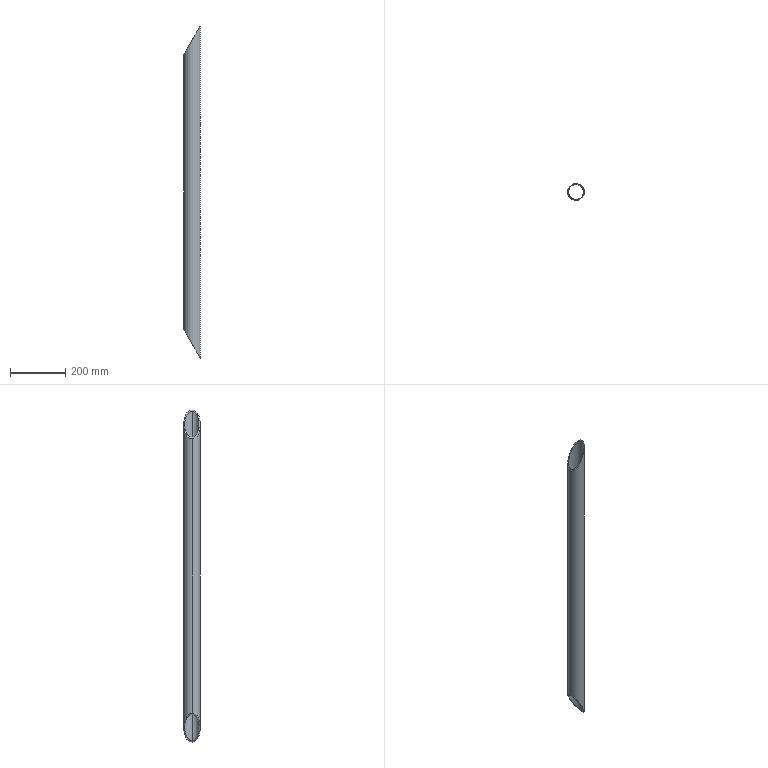Part | SolidWorks | features BaseBody 1, HoleWzd 1 | 1 solid | 6 faces | box 60.3 x 60.3 x 1200 mm | volume 628920 mm3 | cylinder 4 | plane 2 | commonest cylinder face diameters 53.9 x2 60.3 x2
STEP:
#1=CARTESIAN_POINT('',(-26.95,0.,-501.1));
#2=VERTEX_POINT('',#1);
#3=CARTESIAN_POINT('',(26.95,0.,-594.457));
#4=VERTEX_POINT('',#3);
#5=CARTESIAN_POINT('',(-26.95,0.,-501.1));
#6=CARTESIAN_POINT('',(-26.95,-53.9,-501.1));
#7=CARTESIAN_POINT('',(26.95,-53.9,-594.457));
#8=CARTESIAN_POINT('',(26.95,0.,-594.457));
#9=(BOUNDED_CURVE()B_SPLINE_CURVE(3,(#5,#6,#7,#8),.UNSPECIFIED.,.F.,.T.)B_SPLINE_CURVE_WITH_KNOTS((4,4),(0.,3.142),.UNSPECIFIED.)CURVE()GEOMETRIC_REPRESENTATION_ITEM()RATIONAL_B_SPLINE_CURVE((1.,0.3333,0.3333,1.))REPRESENTATION_ITEM(''));
#10=EDGE_CURVE('',#2,#4,#9,.T.);
#11=ORIENTED_EDGE('',*,*,#10,.F.);
#12=CARTESIAN_POINT('',(-26.95,0.,501.1));
#13=VERTEX_POINT('',#12);
#14=CARTESIAN_POINT('',(-26.95,0.,597.229));
#15=DIRECTION('',(0.,0.,1.));
#16=VECTOR('',#15,1000.);
#17=LINE('',#14,#16);
#18=EDGE_CURVE('',#2,#13,#17,.T.);
#19=ORIENTED_EDGE('',*,*,#18,.T.);
#20=CARTESIAN_POINT('',(26.95,0.,594.457));
#21=VERTEX_POINT('',#20);
#22=CARTESIAN_POINT('',(-26.95,0.,501.1));
#23=CARTESIAN_POINT('',(-26.95,-53.9,501.1));
#24=CARTESIAN_POINT('',(26.95,-53.9,594.457));
#25=CARTESIAN_POINT('',(26.95,0.,594.457));
#26=(BOUNDED_CURVE()B_SPLINE_CURVE(3,(#22,#23,#24,#25),.UNSPECIFIED.,.F.,.T.)B_SPLINE_CURVE_WITH_KNOTS((4,4),(3.142,6.283),.UNSPECIFIED.)CURVE()GEOMETRIC_REPRESENTATION_ITEM()RATIONAL_B_SPLINE_CURVE((1.,0.3333,0.3333,1.))REPRESENTATION_ITEM(''));
#27=EDGE_CURVE('',#13,#21,#26,.T.);
#28=ORIENTED_EDGE('',*,*,#27,.T.);
#29=CARTESIAN_POINT('',(26.95,0.,597.229));
#30=DIRECTION('',(0.,0.,1.));
#31=VECTOR('',#30,1000.);
#32=LINE('',#29,#31);
#33=EDGE_CURVE('',#4,#21,#32,.T.);
#34=ORIENTED_EDGE('',*,*,#33,.F.);
#35=EDGE_LOOP('',(#11,#19,#28,#34));
#36=FACE_OUTER_BOUND('',#35,.T.);
#37=CARTESIAN_POINT('',(0.,0.,597.229));
#38=DIRECTION('',(0.,0.,1.));
#39=DIRECTION('',(1.,0.,0.));
#40=AXIS2_PLACEMENT_3D('',#37,#38,#39);
#41=CYLINDRICAL_SURFACE('',#40,26.95);
#42=ADVANCED_FACE('',(#36),#41,.F.);
#43=CARTESIAN_POINT('',(30.15,0.,600.));
#44=VERTEX_POINT('',#43);
#45=CARTESIAN_POINT('',(-30.15,0.,495.557));
#46=VERTEX_POINT('',#45);
#47=CARTESIAN_POINT('',(30.15,0.,600.));
#48=CARTESIAN_POINT('',(30.15,60.3,600.));
#49=CARTESIAN_POINT('',(-30.15,60.3,495.557));
#50=CARTESIAN_POINT('',(-30.15,0.,495.557));
#51=(BOUNDED_CURVE()B_SPLINE_CURVE(3,(#47,#48,#49,#50),.UNSPECIFIED.,.F.,.T.)B_SPLINE_CURVE_WITH_KNOTS((4,4),(3.142,6.283),.UNSPECIFIED.)CURVE()GEOMETRIC_REPRESENTATION_ITEM()RATIONAL_B_SPLINE_CURVE((1.,0.3333,0.3333,1.))REPRESENTATION_ITEM(''));
#52=EDGE_CURVE('',#44,#46,#51,.T.);
#53=ORIENTED_EDGE('',*,*,#52,.F.);
#54=CARTESIAN_POINT('',(30.15,0.,-600.));
#55=VERTEX_POINT('',#54);
#56=CARTESIAN_POINT('',(30.15,0.,600.));
#57=DIRECTION('',(0.,0.,-1.));
#58=VECTOR('',#57,1000.);
#59=LINE('',#56,#58);
#60=EDGE_CURVE('',#44,#55,#59,.T.);
#61=ORIENTED_EDGE('',*,*,#60,.T.);
#62=CARTESIAN_POINT('',(-30.15,0.,-495.557));
#63=VERTEX_POINT('',#62);
#64=CARTESIAN_POINT('',(30.15,0.,-600.));
#65=CARTESIAN_POINT('',(30.15,60.3,-600.));
#66=CARTESIAN_POINT('',(-30.15,60.3,-495.557));
#67=CARTESIAN_POINT('',(-30.15,0.,-495.557));
#68=(BOUNDED_CURVE()B_SPLINE_CURVE(3,(#64,#65,#66,#67),.UNSPECIFIED.,.F.,.T.)B_SPLINE_CURVE_WITH_KNOTS((4,4),(0.,3.142),.UNSPECIFIED.)CURVE()GEOMETRIC_REPRESENTATION_ITEM()RATIONAL_B_SPLINE_CURVE((1.,0.3333,0.3333,1.))REPRESENTATION_ITEM(''));
#69=EDGE_CURVE('',#55,#63,#68,.T.);
#70=ORIENTED_EDGE('',*,*,#69,.T.);
#71=CARTESIAN_POINT('',(-30.15,0.,600.));
#72=DIRECTION('',(0.,0.,-1.));
#73=VECTOR('',#72,1000.);
#74=LINE('',#71,#73);
#75=EDGE_CURVE('',#46,#63,#74,.T.);
#76=ORIENTED_EDGE('',*,*,#75,.F.);
#77=EDGE_LOOP('',(#53,#61,#70,#76));
#78=FACE_OUTER_BOUND('',#77,.T.);
#79=CARTESIAN_POINT('',(0.,0.,600.));
#80=DIRECTION('',(0.,0.,-1.));
#81=DIRECTION('',(-1.,0.,0.));
#82=AXIS2_PLACEMENT_3D('',#79,#80,#81);
#83=CYLINDRICAL_SURFACE('',#82,30.15);
#84=ADVANCED_FACE('',(#78),#83,.T.);
#85=ORIENTED_EDGE('',*,*,#60,.F.);
#86=CARTESIAN_POINT('',(-30.15,0.,495.557));
#87=CARTESIAN_POINT('',(-30.15,-60.3,495.557));
#88=CARTESIAN_POINT('',(30.15,-60.3,600.));
#89=CARTESIAN_POINT('',(30.15,0.,600.));
#90=(BOUNDED_CURVE()B_SPLINE_CURVE(3,(#86,#87,#88,#89),.UNSPECIFIED.,.F.,.T.)B_SPLINE_CURVE_WITH_KNOTS((4,4),(0.,3.142),.UNSPECIFIED.)CURVE()GEOMETRIC_REPRESENTATION_ITEM()RATIONAL_B_SPLINE_CURVE((1.,0.3333,0.3333,1.))REPRESENTATION_ITEM(''));
#91=EDGE_CURVE('',#46,#44,#90,.T.);
#92=ORIENTED_EDGE('',*,*,#91,.F.);
#93=ORIENTED_EDGE('',*,*,#75,.T.);
#94=CARTESIAN_POINT('',(-30.15,0.,-495.557));
#95=CARTESIAN_POINT('',(-30.15,-60.3,-495.557));
#96=CARTESIAN_POINT('',(30.15,-60.3,-600.));
#97=CARTESIAN_POINT('',(30.15,0.,-600.));
#98=(BOUNDED_CURVE()B_SPLINE_CURVE(3,(#94,#95,#96,#97),.UNSPECIFIED.,.F.,.T.)B_SPLINE_CURVE_WITH_KNOTS((4,4),(3.142,6.283),.UNSPECIFIED.)CURVE()GEOMETRIC_REPRESENTATION_ITEM()RATIONAL_B_SPLINE_CURVE((1.,0.3333,0.3333,1.))REPRESENTATION_ITEM(''));
#99=EDGE_CURVE('',#63,#55,#98,.T.);
#100=ORIENTED_EDGE('',*,*,#99,.T.);
#101=EDGE_LOOP('',(#85,#92,#93,#100));
#102=FACE_OUTER_BOUND('',#101,.T.);
#103=CARTESIAN_POINT('',(0.,0.,600.));
#104=DIRECTION('',(0.,0.,-1.));
#105=DIRECTION('',(-1.,0.,0.));
#106=AXIS2_PLACEMENT_3D('',#103,#104,#105);
#107=CYLINDRICAL_SURFACE('',#106,30.15);
#108=ADVANCED_FACE('',(#102),#107,.T.);
#109=CARTESIAN_POINT('',(26.95,0.,-594.457));
#110=CARTESIAN_POINT('',(26.95,53.9,-594.457));
#111=CARTESIAN_POINT('',(-26.95,53.9,-501.1));
#112=CARTESIAN_POINT('',(-26.95,0.,-501.1));
#113=(BOUNDED_CURVE()B_SPLINE_CURVE(3,(#109,#110,#111,#112),.UNSPECIFIED.,.F.,.T.)B_SPLINE_CURVE_WITH_KNOTS((4,4),(3.142,6.283),.UNSPECIFIED.)CURVE()GEOMETRIC_REPRESENTATION_ITEM()RATIONAL_B_SPLINE_CURVE((1.,0.3333,0.3333,1.))REPRESENTATION_ITEM(''));
#114=EDGE_CURVE('',#4,#2,#113,.T.);
#115=ORIENTED_EDGE('',*,*,#114,.T.);
#116=ORIENTED_EDGE('',*,*,#10,.T.);
#117=EDGE_LOOP('',(#115,#116));
#118=FACE_BOUND('',#117,.T.);
#119=ORIENTED_EDGE('',*,*,#99,.F.);
#120=ORIENTED_EDGE('',*,*,#69,.F.);
#121=EDGE_LOOP('',(#119,#120));
#122=FACE_OUTER_BOUND('',#121,.T.);
#123=CARTESIAN_POINT('',(30.15,-50.,-600.));
#124=DIRECTION('',(0.866,0.,0.5));
#125=DIRECTION('',(0.5,0.,-0.866));
#126=AXIS2_PLACEMENT_3D('',#123,#124,#125);
#127=PLANE('',#126);
#128=ADVANCED_FACE('',(#118,#122),#127,.F.);
#129=CARTESIAN_POINT('',(26.95,0.,594.457));
#130=CARTESIAN_POINT('',(26.95,53.9,594.457));
#131=CARTESIAN_POINT('',(-26.95,53.9,501.1));
#132=CARTESIAN_POINT('',(-26.95,0.,501.1));
#133=(BOUNDED_CURVE()B_SPLINE_CURVE(3,(#129,#130,#131,#132),.UNSPECIFIED.,.F.,.T.)B_SPLINE_CURVE_WITH_KNOTS((4,4),(0.,3.142),.UNSPECIFIED.)CURVE()GEOMETRIC_REPRESENTATION_ITEM()RATIONAL_B_SPLINE_CURVE((1.,0.3333,0.3333,1.))REPRESENTATION_ITEM(''));
#134=EDGE_CURVE('',#21,#13,#133,.T.);
#135=ORIENTED_EDGE('',*,*,#134,.F.);
#136=ORIENTED_EDGE('',*,*,#27,.F.);
#137=EDGE_LOOP('',(#135,#136));
#138=FACE_BOUND('',#137,.T.);
#139=ORIENTED_EDGE('',*,*,#91,.T.);
#140=ORIENTED_EDGE('',*,*,#52,.T.);
#141=EDGE_LOOP('',(#139,#140));
#142=FACE_OUTER_BOUND('',#141,.T.);
#143=CARTESIAN_POINT('',(30.15,-50.,600.));
#144=DIRECTION('',(-0.866,0.,0.5));
#145=DIRECTION('',(0.5,0.,0.866));
#146=AXIS2_PLACEMENT_3D('',#143,#144,#145);
#147=PLANE('',#146);
#148=ADVANCED_FACE('',(#138,#142),#147,.T.);
#149=ORIENTED_EDGE('',*,*,#18,.F.);
#150=ORIENTED_EDGE('',*,*,#114,.F.);
#151=ORIENTED_EDGE('',*,*,#33,.T.);
#152=ORIENTED_EDGE('',*,*,#134,.T.);
#153=EDGE_LOOP('',(#149,#150,#151,#152));
#154=FACE_OUTER_BOUND('',#153,.T.);
#155=CARTESIAN_POINT('',(0.,0.,597.229));
#156=DIRECTION('',(0.,0.,1.));
#157=DIRECTION('',(1.,0.,0.));
#158=AXIS2_PLACEMENT_3D('',#155,#156,#157);
#159=CYLINDRICAL_SURFACE('',#158,26.95);
#160=ADVANCED_FACE('',(#154),#159,.F.);
#161=CLOSED_SHELL('',(#42,#84,#108,#128,#148,#160));
#162=MANIFOLD_SOLID_BREP('',#161);
#163=CARTESIAN_POINT('',(0.,0.,0.));
#164=DIRECTION('',(0.,0.,1.));
#165=DIRECTION('',(1.,0.,0.));
#166=AXIS2_PLACEMENT_3D('',#163,#164,#165);
#167=(LENGTH_UNIT()NAMED_UNIT(*)SI_UNIT(.MILLI.,.METRE.));
#168=UNCERTAINTY_MEASURE_WITH_UNIT(LENGTH_MEASURE(0.00001),#167,'','');
#169=(NAMED_UNIT(*)PLANE_ANGLE_UNIT()SI_UNIT($,.RADIAN.));
#170=(NAMED_UNIT(*)SI_UNIT($,.STERADIAN.)SOLID_ANGLE_UNIT());
#171=(GEOMETRIC_REPRESENTATION_CONTEXT(3)GLOBAL_UNCERTAINTY_ASSIGNED_CONTEXT((#168))GLOBAL_UNIT_ASSIGNED_CONTEXT((#167,#169,#170))REPRESENTATION_CONTEXT('',''));
#172=ADVANCED_BREP_SHAPE_REPRESENTATION('',(#162,#166),#171);